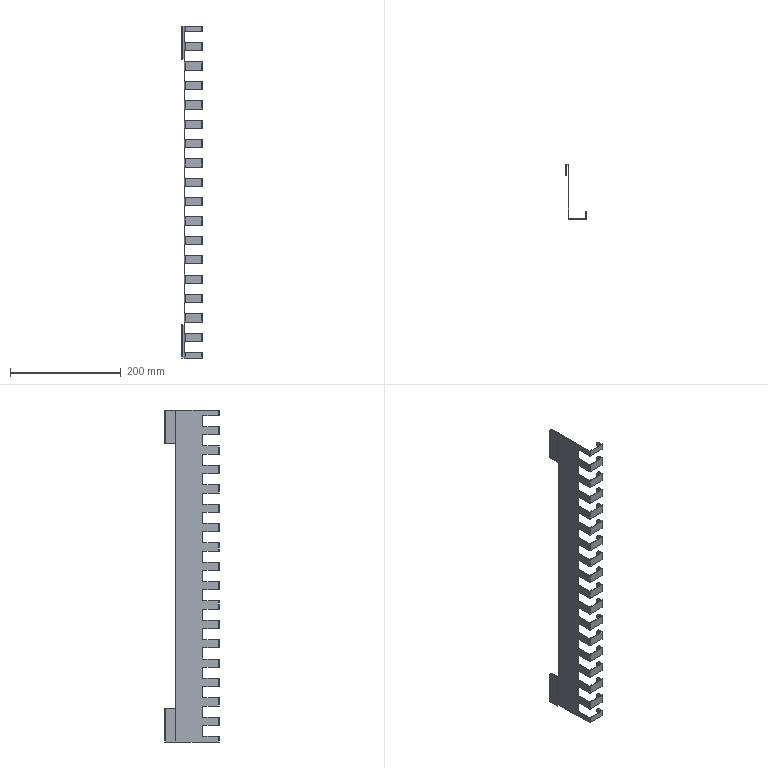Part | SolidWorks | features ICE 4, LPattern 2, FlatPattern 1, MirrorPattern 1, SMBaseFlange 1, SheetMetal 1 | 1 solid | 398 faces | box 37.5 x 99 x 600 mm | volume 79648 mm3 | plane 300 | cylinder 98 | commonest cylinder face diameters 0.4 x40 3.4 x40 15.296 x16 10 x2